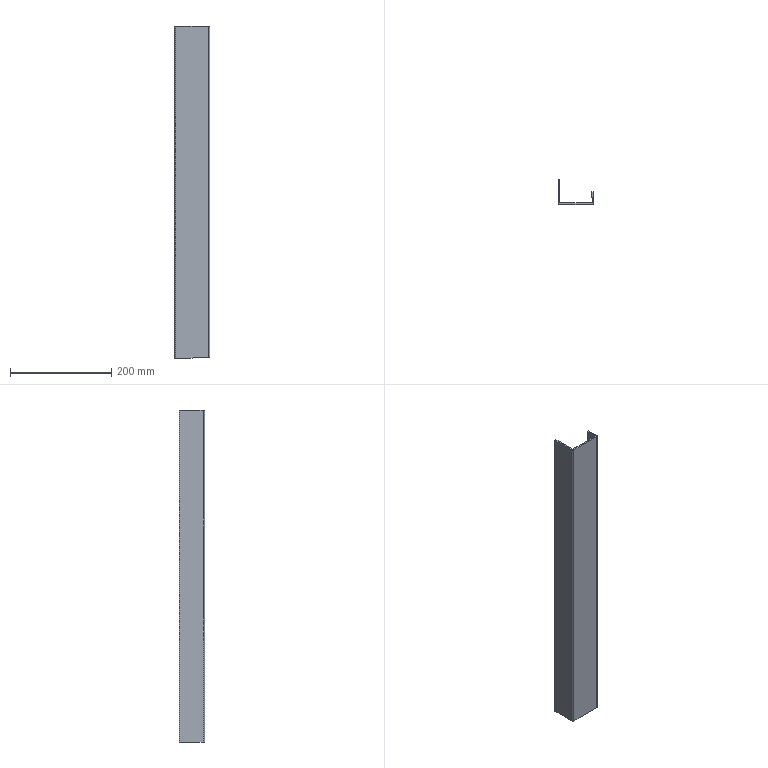Part | SolidWorks | 1 solid | 22 faces | box 69.995 x 50 x 656 mm | volume 270732 mm3 | plane 18 | cylinder 4 | commonest cylinder face diameters 0.2 x2 6.2 x2
STEP:
#1=CARTESIAN_POINT('',(31.895,-3.,-328.));
#2=VERTEX_POINT('',#1);
#3=CARTESIAN_POINT('',(31.895,-3.,328.));
#4=VERTEX_POINT('',#3);
#5=CARTESIAN_POINT('',(31.895,-3.,-328.));
#6=DIRECTION('',(0.,0.,1.));
#7=VECTOR('',#6,1000.);
#8=LINE('',#5,#7);
#9=EDGE_CURVE('',#2,#4,#8,.T.);
#10=ORIENTED_EDGE('',*,*,#9,.T.);
#11=CARTESIAN_POINT('',(-31.9,-3.,328.));
#12=VERTEX_POINT('',#11);
#13=CARTESIAN_POINT('',(35.,-3.,328.));
#14=DIRECTION('',(1.,0.,0.));
#15=VECTOR('',#14,1000.);
#16=LINE('',#13,#15);
#17=EDGE_CURVE('',#12,#4,#16,.T.);
#18=ORIENTED_EDGE('',*,*,#17,.F.);
#19=CARTESIAN_POINT('',(-31.9,-3.,-328.));
#20=VERTEX_POINT('',#19);
#21=CARTESIAN_POINT('',(-31.9,-3.,328.));
#22=DIRECTION('',(0.,0.,-1.));
#23=VECTOR('',#22,1000.);
#24=LINE('',#21,#23);
#25=EDGE_CURVE('',#12,#20,#24,.T.);
#26=ORIENTED_EDGE('',*,*,#25,.T.);
#27=CARTESIAN_POINT('',(35.,-3.,-328.));
#28=DIRECTION('',(-1.,0.,0.));
#29=VECTOR('',#28,1000.);
#30=LINE('',#27,#29);
#31=EDGE_CURVE('',#2,#20,#30,.T.);
#32=ORIENTED_EDGE('',*,*,#31,.F.);
#33=EDGE_LOOP('',(#10,#18,#26,#32));
#34=FACE_OUTER_BOUND('',#33,.T.);
#35=CARTESIAN_POINT('',(0.,-3.,0.));
#36=DIRECTION('',(0.,1.,0.));
#37=DIRECTION('',(0.,0.,1.));
#38=AXIS2_PLACEMENT_3D('',#35,#36,#37);
#39=PLANE('',#38);
#40=ADVANCED_FACE('',(#34),#39,.F.);
#41=CARTESIAN_POINT('',(-31.9,0.,328.));
#42=VERTEX_POINT('',#41);
#43=CARTESIAN_POINT('',(31.895,0.,328.));
#44=VERTEX_POINT('',#43);
#45=CARTESIAN_POINT('',(35.,0.,328.));
#46=DIRECTION('',(1.,0.,0.));
#47=VECTOR('',#46,1000.);
#48=LINE('',#45,#47);
#49=EDGE_CURVE('',#42,#44,#48,.T.);
#50=ORIENTED_EDGE('',*,*,#49,.T.);
#51=CARTESIAN_POINT('',(31.895,0.,-328.));
#52=VERTEX_POINT('',#51);
#53=CARTESIAN_POINT('',(31.895,0.,-328.));
#54=DIRECTION('',(0.,0.,1.));
#55=VECTOR('',#54,1000.);
#56=LINE('',#53,#55);
#57=EDGE_CURVE('',#52,#44,#56,.T.);
#58=ORIENTED_EDGE('',*,*,#57,.F.);
#59=CARTESIAN_POINT('',(-31.9,0.,-328.));
#60=VERTEX_POINT('',#59);
#61=CARTESIAN_POINT('',(35.,0.,-328.));
#62=DIRECTION('',(-1.,0.,0.));
#63=VECTOR('',#62,1000.);
#64=LINE('',#61,#63);
#65=EDGE_CURVE('',#52,#60,#64,.T.);
#66=ORIENTED_EDGE('',*,*,#65,.T.);
#67=CARTESIAN_POINT('',(-31.9,0.,328.));
#68=DIRECTION('',(0.,0.,-1.));
#69=VECTOR('',#68,1000.);
#70=LINE('',#67,#69);
#71=EDGE_CURVE('',#42,#60,#70,.T.);
#72=ORIENTED_EDGE('',*,*,#71,.F.);
#73=EDGE_LOOP('',(#50,#58,#66,#72));
#74=FACE_OUTER_BOUND('',#73,.T.);
#75=CARTESIAN_POINT('',(0.,0.,0.));
#76=DIRECTION('',(0.,1.,0.));
#77=DIRECTION('',(0.,0.,1.));
#78=AXIS2_PLACEMENT_3D('',#75,#76,#77);
#79=PLANE('',#78);
#80=ADVANCED_FACE('',(#74),#79,.T.);
#81=ORIENTED_EDGE('',*,*,#65,.F.);
#82=CARTESIAN_POINT('',(31.895,0.,-328.));
#83=DIRECTION('',(0.,-1.,0.));
#84=VECTOR('',#83,1000.);
#85=LINE('',#82,#84);
#86=EDGE_CURVE('',#52,#2,#85,.T.);
#87=ORIENTED_EDGE('',*,*,#86,.T.);
#88=ORIENTED_EDGE('',*,*,#31,.T.);
#89=CARTESIAN_POINT('',(-31.9,0.,-328.));
#90=DIRECTION('',(0.,-1.,0.));
#91=VECTOR('',#90,1000.);
#92=LINE('',#89,#91);
#93=EDGE_CURVE('',#60,#20,#92,.T.);
#94=ORIENTED_EDGE('',*,*,#93,.F.);
#95=EDGE_LOOP('',(#81,#87,#88,#94));
#96=FACE_OUTER_BOUND('',#95,.T.);
#97=CARTESIAN_POINT('',(35.,-3.,-328.));
#98=DIRECTION('',(0.,0.,-1.));
#99=DIRECTION('',(-1.,0.,0.));
#100=AXIS2_PLACEMENT_3D('',#97,#98,#99);
#101=PLANE('',#100);
#102=ADVANCED_FACE('',(#96),#101,.T.);
#103=CARTESIAN_POINT('',(31.895,0.,328.));
#104=DIRECTION('',(0.,-1.,0.));
#105=VECTOR('',#104,1000.);
#106=LINE('',#103,#105);
#107=EDGE_CURVE('',#44,#4,#106,.T.);
#108=ORIENTED_EDGE('',*,*,#107,.F.);
#109=ORIENTED_EDGE('',*,*,#49,.F.);
#110=CARTESIAN_POINT('',(-31.9,0.,328.));
#111=DIRECTION('',(0.,-1.,0.));
#112=VECTOR('',#111,1000.);
#113=LINE('',#110,#112);
#114=EDGE_CURVE('',#42,#12,#113,.T.);
#115=ORIENTED_EDGE('',*,*,#114,.T.);
#116=ORIENTED_EDGE('',*,*,#17,.T.);
#117=EDGE_LOOP('',(#108,#109,#115,#116));
#118=FACE_OUTER_BOUND('',#117,.T.);
#119=CARTESIAN_POINT('',(35.,-3.,328.));
#120=DIRECTION('',(0.,0.,1.));
#121=DIRECTION('',(1.,0.,0.));
#122=AXIS2_PLACEMENT_3D('',#119,#120,#121);
#123=PLANE('',#122);
#124=ADVANCED_FACE('',(#118),#123,.T.);
#125=CARTESIAN_POINT('',(-32.,0.1,-328.));
#126=VERTEX_POINT('',#125);
#127=CARTESIAN_POINT('',(-35.,0.1,-328.));
#128=VERTEX_POINT('',#127);
#129=CARTESIAN_POINT('',(-35.,0.1,-328.));
#130=DIRECTION('',(-1.,0.,0.));
#131=VECTOR('',#130,1000.);
#132=LINE('',#129,#131);
#133=EDGE_CURVE('',#126,#128,#132,.T.);
#134=ORIENTED_EDGE('',*,*,#133,.F.);
#135=CARTESIAN_POINT('',(-31.9,0.1,-328.));
#136=DIRECTION('',(0.,0.,-1.));
#137=DIRECTION('',(1.,0.,0.));
#138=AXIS2_PLACEMENT_3D('',#135,#136,#137);
#139=CIRCLE('',#138,0.1);
#140=EDGE_CURVE('',#60,#126,#139,.T.);
#141=ORIENTED_EDGE('',*,*,#140,.F.);
#142=ORIENTED_EDGE('',*,*,#93,.T.);
#143=CARTESIAN_POINT('',(-31.9,0.1,-328.));
#144=DIRECTION('',(0.,0.,-1.));
#145=DIRECTION('',(1.,0.,0.));
#146=AXIS2_PLACEMENT_3D('',#143,#144,#145);
#147=CIRCLE('',#146,3.1);
#148=EDGE_CURVE('',#20,#128,#147,.T.);
#149=ORIENTED_EDGE('',*,*,#148,.T.);
#150=EDGE_LOOP('',(#134,#141,#142,#149));
#151=FACE_OUTER_BOUND('',#150,.T.);
#152=CARTESIAN_POINT('',(-31.9,0.1,-328.));
#153=DIRECTION('',(0.,0.,-1.));
#154=DIRECTION('',(-1.,0.,0.));
#155=AXIS2_PLACEMENT_3D('',#152,#153,#154);
#156=PLANE('',#155);
#157=ADVANCED_FACE('',(#151),#156,.T.);
#158=CARTESIAN_POINT('',(-32.,0.1,328.));
#159=VERTEX_POINT('',#158);
#160=CARTESIAN_POINT('',(-31.9,0.1,328.));
#161=DIRECTION('',(0.,0.,1.));
#162=DIRECTION('',(1.,0.,0.));
#163=AXIS2_PLACEMENT_3D('',#160,#161,#162);
#164=CIRCLE('',#163,0.1);
#165=EDGE_CURVE('',#159,#42,#164,.T.);
#166=ORIENTED_EDGE('',*,*,#165,.F.);
#167=CARTESIAN_POINT('',(-35.,0.1,328.));
#168=VERTEX_POINT('',#167);
#169=CARTESIAN_POINT('',(-32.,0.1,328.));
#170=DIRECTION('',(-1.,0.,0.));
#171=VECTOR('',#170,1000.);
#172=LINE('',#169,#171);
#173=EDGE_CURVE('',#159,#168,#172,.T.);
#174=ORIENTED_EDGE('',*,*,#173,.T.);
#175=CARTESIAN_POINT('',(-31.9,0.1,328.));
#176=DIRECTION('',(0.,0.,1.));
#177=DIRECTION('',(1.,0.,0.));
#178=AXIS2_PLACEMENT_3D('',#175,#176,#177);
#179=CIRCLE('',#178,3.1);
#180=EDGE_CURVE('',#168,#12,#179,.T.);
#181=ORIENTED_EDGE('',*,*,#180,.T.);
#182=ORIENTED_EDGE('',*,*,#114,.F.);
#183=EDGE_LOOP('',(#166,#174,#181,#182));
#184=FACE_OUTER_BOUND('',#183,.T.);
#185=CARTESIAN_POINT('',(-31.9,0.1,328.));
#186=DIRECTION('',(0.,0.,-1.));
#187=DIRECTION('',(-1.,0.,0.));
#188=AXIS2_PLACEMENT_3D('',#185,#186,#187);
#189=PLANE('',#188);
#190=ADVANCED_FACE('',(#184),#189,.F.);
#191=ORIENTED_EDGE('',*,*,#25,.F.);
#192=ORIENTED_EDGE('',*,*,#180,.F.);
#193=CARTESIAN_POINT('',(-35.,0.1,-328.));
#194=DIRECTION('',(0.,0.,-1.));
#195=VECTOR('',#194,1000.);
#196=LINE('',#193,#195);
#197=EDGE_CURVE('',#168,#128,#196,.T.);
#198=ORIENTED_EDGE('',*,*,#197,.T.);
#199=ORIENTED_EDGE('',*,*,#148,.F.);
#200=EDGE_LOOP('',(#191,#192,#198,#199));
#201=FACE_OUTER_BOUND('',#200,.T.);
#202=CARTESIAN_POINT('',(-31.9,0.1,328.));
#203=DIRECTION('',(0.,0.,1.));
#204=DIRECTION('',(-1.,0.,0.));
#205=AXIS2_PLACEMENT_3D('',#202,#203,#204);
#206=CYLINDRICAL_SURFACE('',#205,3.1);
#207=ADVANCED_FACE('',(#201),#206,.T.);
#208=ORIENTED_EDGE('',*,*,#71,.T.);
#209=ORIENTED_EDGE('',*,*,#140,.T.);
#210=CARTESIAN_POINT('',(-32.,0.1,-328.));
#211=DIRECTION('',(0.,0.,1.));
#212=VECTOR('',#211,1000.);
#213=LINE('',#210,#212);
#214=EDGE_CURVE('',#126,#159,#213,.T.);
#215=ORIENTED_EDGE('',*,*,#214,.T.);
#216=ORIENTED_EDGE('',*,*,#165,.T.);
#217=EDGE_LOOP('',(#208,#209,#215,#216));
#218=FACE_OUTER_BOUND('',#217,.T.);
#219=CARTESIAN_POINT('',(-31.9,0.1,328.));
#220=DIRECTION('',(0.,0.,1.));
#221=DIRECTION('',(-1.,0.,0.));
#222=AXIS2_PLACEMENT_3D('',#219,#220,#221);
#223=CYLINDRICAL_SURFACE('',#222,0.1);
#224=ADVANCED_FACE('',(#218),#223,.F.);
#225=ORIENTED_EDGE('',*,*,#133,.T.);
#226=CARTESIAN_POINT('',(-35.,47.,-328.));
#227=VERTEX_POINT('',#226);
#228=CARTESIAN_POINT('',(-35.,0.,-328.));
#229=DIRECTION('',(0.,-1.,0.));
#230=VECTOR('',#229,1000.);
#231=LINE('',#228,#230);
#232=EDGE_CURVE('',#227,#128,#231,.T.);
#233=ORIENTED_EDGE('',*,*,#232,.F.);
#234=CARTESIAN_POINT('',(-32.,47.,-328.));
#235=VERTEX_POINT('',#234);
#236=CARTESIAN_POINT('',(-35.,47.,-328.));
#237=DIRECTION('',(1.,0.,0.));
#238=VECTOR('',#237,1000.);
#239=LINE('',#236,#238);
#240=EDGE_CURVE('',#227,#235,#239,.T.);
#241=ORIENTED_EDGE('',*,*,#240,.T.);
#242=CARTESIAN_POINT('',(-32.,0.,-328.));
#243=DIRECTION('',(0.,-1.,0.));
#244=VECTOR('',#243,1000.);
#245=LINE('',#242,#244);
#246=EDGE_CURVE('',#235,#126,#245,.T.);
#247=ORIENTED_EDGE('',*,*,#246,.T.);
#248=EDGE_LOOP('',(#225,#233,#241,#247));
#249=FACE_OUTER_BOUND('',#248,.T.);
#250=CARTESIAN_POINT('',(-35.,0.,-328.));
#251=DIRECTION('',(0.,0.,1.));
#252=DIRECTION('',(1.,0.,0.));
#253=AXIS2_PLACEMENT_3D('',#250,#251,#252);
#254=PLANE('',#253);
#255=ADVANCED_FACE('',(#249),#254,.F.);
#256=ORIENTED_EDGE('',*,*,#173,.F.);
#257=CARTESIAN_POINT('',(-32.,47.,328.));
#258=VERTEX_POINT('',#257);
#259=CARTESIAN_POINT('',(-32.,47.,328.));
#260=DIRECTION('',(0.,1.,0.));
#261=VECTOR('',#260,1000.);
#262=LINE('',#259,#261);
#263=EDGE_CURVE('',#159,#258,#262,.T.);
#264=ORIENTED_EDGE('',*,*,#263,.T.);
#265=CARTESIAN_POINT('',(-35.,47.,328.));
#266=VERTEX_POINT('',#265);
#267=CARTESIAN_POINT('',(-35.,47.,328.));
#268=DIRECTION('',(1.,0.,0.));
#269=VECTOR('',#268,1000.);
#270=LINE('',#267,#269);
#271=EDGE_CURVE('',#266,#258,#270,.T.);
#272=ORIENTED_EDGE('',*,*,#271,.F.);
#273=CARTESIAN_POINT('',(-35.,0.,328.));
#274=DIRECTION('',(0.,1.,0.));
#275=VECTOR('',#274,1000.);
#276=LINE('',#273,#275);
#277=EDGE_CURVE('',#168,#266,#276,.T.);
#278=ORIENTED_EDGE('',*,*,#277,.F.);
#279=EDGE_LOOP('',(#256,#264,#272,#278));
#280=FACE_OUTER_BOUND('',#279,.T.);
#281=CARTESIAN_POINT('',(-35.,47.,328.));
#282=DIRECTION('',(0.,0.,-1.));
#283=DIRECTION('',(0.,1.,0.));
#284=AXIS2_PLACEMENT_3D('',#281,#282,#283);
#285=PLANE('',#284);
#286=ADVANCED_FACE('',(#280),#285,.F.);
#287=ORIENTED_EDGE('',*,*,#197,.F.);
#288=ORIENTED_EDGE('',*,*,#277,.T.);
#289=CARTESIAN_POINT('',(-35.,47.,0.));
#290=DIRECTION('',(0.,0.,-1.));
#291=VECTOR('',#290,1000.);
#292=LINE('',#289,#291);
#293=EDGE_CURVE('',#266,#227,#292,.T.);
#294=ORIENTED_EDGE('',*,*,#293,.T.);
#295=ORIENTED_EDGE('',*,*,#232,.T.);
#296=EDGE_LOOP('',(#287,#288,#294,#295));
#297=FACE_OUTER_BOUND('',#296,.T.);
#298=CARTESIAN_POINT('',(-35.,0.,0.));
#299=DIRECTION('',(1.,0.,0.));
#300=DIRECTION('',(0.,1.,0.));
#301=AXIS2_PLACEMENT_3D('',#298,#299,#300);
#302=PLANE('',#301);
#303=ADVANCED_FACE('',(#297),#302,.F.);
#304=ORIENTED_EDGE('',*,*,#263,.F.);
#305=ORIENTED_EDGE('',*,*,#214,.F.);
#306=ORIENTED_EDGE('',*,*,#246,.F.);
#307=CARTESIAN_POINT('',(-32.,47.,-328.));
#308=DIRECTION('',(0.,0.,-1.));
#309=VECTOR('',#308,1000.);
#310=LINE('',#307,#309);
#311=EDGE_CURVE('',#258,#235,#310,.T.);
#312=ORIENTED_EDGE('',*,*,#311,.F.);
#313=EDGE_LOOP('',(#304,#305,#306,#312));
#314=FACE_OUTER_BOUND('',#313,.T.);
#315=CARTESIAN_POINT('',(-32.,0.,0.));
#316=DIRECTION('',(1.,0.,0.));
#317=DIRECTION('',(0.,1.,0.));
#318=AXIS2_PLACEMENT_3D('',#315,#316,#317);
#319=PLANE('',#318);
#320=ADVANCED_FACE('',(#314),#319,.T.);
#321=ORIENTED_EDGE('',*,*,#311,.T.);
#322=ORIENTED_EDGE('',*,*,#240,.F.);
#323=ORIENTED_EDGE('',*,*,#293,.F.);
#324=ORIENTED_EDGE('',*,*,#271,.T.);
#325=EDGE_LOOP('',(#321,#322,#323,#324));
#326=FACE_OUTER_BOUND('',#325,.T.);
#327=CARTESIAN_POINT('',(-35.,47.,-328.));
#328=DIRECTION('',(0.,-1.,0.));
#329=DIRECTION('',(1.,0.,0.));
#330=AXIS2_PLACEMENT_3D('',#327,#328,#329);
#331=PLANE('',#330);
#332=ADVANCED_FACE('',(#326),#331,.F.);
#333=CARTESIAN_POINT('',(31.995,0.1035,328.));
#334=VERTEX_POINT('',#333);
#335=CARTESIAN_POINT('',(34.993,0.2082,328.));
#336=VERTEX_POINT('',#335);
#337=CARTESIAN_POINT('',(34.993,0.2082,328.));
#338=DIRECTION('',(0.9994,0.0349,0.));
#339=VECTOR('',#338,1000.);
#340=LINE('',#337,#339);
#341=EDGE_CURVE('',#334,#336,#340,.T.);
#342=ORIENTED_EDGE('',*,*,#341,.F.);
#343=CARTESIAN_POINT('',(31.895,0.1,328.));
#344=DIRECTION('',(0.,0.,1.));
#345=DIRECTION('',(-1.,0.,0.));
#346=AXIS2_PLACEMENT_3D('',#343,#344,#345);
#347=CIRCLE('',#346,0.1);
#348=EDGE_CURVE('',#44,#334,#347,.T.);
#349=ORIENTED_EDGE('',*,*,#348,.F.);
#350=ORIENTED_EDGE('',*,*,#107,.T.);
#351=CARTESIAN_POINT('',(31.895,0.1,328.));
#352=DIRECTION('',(0.,0.,1.));
#353=DIRECTION('',(-1.,0.,0.));
#354=AXIS2_PLACEMENT_3D('',#351,#352,#353);
#355=CIRCLE('',#354,3.1);
#356=EDGE_CURVE('',#4,#336,#355,.T.);
#357=ORIENTED_EDGE('',*,*,#356,.T.);
#358=EDGE_LOOP('',(#342,#349,#350,#357));
#359=FACE_OUTER_BOUND('',#358,.T.);
#360=CARTESIAN_POINT('',(31.895,0.1,328.));
#361=DIRECTION('',(0.,0.,1.));
#362=DIRECTION('',(1.,0.,0.));
#363=AXIS2_PLACEMENT_3D('',#360,#361,#362);
#364=PLANE('',#363);
#365=ADVANCED_FACE('',(#359),#364,.T.);
#366=CARTESIAN_POINT('',(31.995,0.1035,-328.));
#367=VERTEX_POINT('',#366);
#368=CARTESIAN_POINT('',(31.895,0.1,-328.));
#369=DIRECTION('',(0.,0.,-1.));
#370=DIRECTION('',(-1.,0.,0.));
#371=AXIS2_PLACEMENT_3D('',#368,#369,#370);
#372=CIRCLE('',#371,0.1);
#373=EDGE_CURVE('',#367,#52,#372,.T.);
#374=ORIENTED_EDGE('',*,*,#373,.F.);
#375=CARTESIAN_POINT('',(34.993,0.2082,-328.));
#376=VERTEX_POINT('',#375);
#377=CARTESIAN_POINT('',(31.995,0.1035,-328.));
#378=DIRECTION('',(0.9994,0.0349,0.));
#379=VECTOR('',#378,1000.);
#380=LINE('',#377,#379);
#381=EDGE_CURVE('',#367,#376,#380,.T.);
#382=ORIENTED_EDGE('',*,*,#381,.T.);
#383=CARTESIAN_POINT('',(31.895,0.1,-328.));
#384=DIRECTION('',(0.,0.,-1.));
#385=DIRECTION('',(-1.,0.,0.));
#386=AXIS2_PLACEMENT_3D('',#383,#384,#385);
#387=CIRCLE('',#386,3.1);
#388=EDGE_CURVE('',#376,#2,#387,.T.);
#389=ORIENTED_EDGE('',*,*,#388,.T.);
#390=ORIENTED_EDGE('',*,*,#86,.F.);
#391=EDGE_LOOP('',(#374,#382,#389,#390));
#392=FACE_OUTER_BOUND('',#391,.T.);
#393=CARTESIAN_POINT('',(31.895,0.1,-328.));
#394=DIRECTION('',(0.,0.,1.));
#395=DIRECTION('',(1.,0.,0.));
#396=AXIS2_PLACEMENT_3D('',#393,#394,#395);
#397=PLANE('',#396);
#398=ADVANCED_FACE('',(#392),#397,.F.);
#399=ORIENTED_EDGE('',*,*,#9,.F.);
#400=ORIENTED_EDGE('',*,*,#388,.F.);
#401=CARTESIAN_POINT('',(34.993,0.2082,328.));
#402=DIRECTION('',(0.,0.,1.));
#403=VECTOR('',#402,1000.);
#404=LINE('',#401,#403);
#405=EDGE_CURVE('',#376,#336,#404,.T.);
#406=ORIENTED_EDGE('',*,*,#405,.T.);
#407=ORIENTED_EDGE('',*,*,#356,.F.);
#408=EDGE_LOOP('',(#399,#400,#406,#407));
#409=FACE_OUTER_BOUND('',#408,.T.);
#410=CARTESIAN_POINT('',(31.895,0.1,-328.));
#411=DIRECTION('',(0.,0.,-1.));
#412=DIRECTION('',(0.9994,0.0349,0.));
#413=AXIS2_PLACEMENT_3D('',#410,#411,#412);
#414=CYLINDRICAL_SURFACE('',#413,3.1);
#415=ADVANCED_FACE('',(#409),#414,.T.);
#416=ORIENTED_EDGE('',*,*,#57,.T.);
#417=ORIENTED_EDGE('',*,*,#348,.T.);
#418=CARTESIAN_POINT('',(31.995,0.1035,328.));
#419=DIRECTION('',(0.,0.,-1.));
#420=VECTOR('',#419,1000.);
#421=LINE('',#418,#420);
#422=EDGE_CURVE('',#334,#367,#421,.T.);
#423=ORIENTED_EDGE('',*,*,#422,.T.);
#424=ORIENTED_EDGE('',*,*,#373,.T.);
#425=EDGE_LOOP('',(#416,#417,#423,#424));
#426=FACE_OUTER_BOUND('',#425,.T.);
#427=CARTESIAN_POINT('',(31.895,0.1,-328.));
#428=DIRECTION('',(0.,0.,-1.));
#429=DIRECTION('',(0.9994,0.0349,0.));
#430=AXIS2_PLACEMENT_3D('',#427,#428,#429);
#431=CYLINDRICAL_SURFACE('',#430,0.1);
#432=ADVANCED_FACE('',(#426),#431,.F.);
#433=ORIENTED_EDGE('',*,*,#381,.F.);
#434=CARTESIAN_POINT('',(31.234,21.88,-328.));
#435=VERTEX_POINT('',#434);
#436=CARTESIAN_POINT('',(31.234,21.88,-328.));
#437=DIRECTION('',(-0.0349,0.9994,0.));
#438=VECTOR('',#437,1000.);
#439=LINE('',#436,#438);
#440=EDGE_CURVE('',#367,#435,#439,.T.);
#441=ORIENTED_EDGE('',*,*,#440,.T.);
#442=CARTESIAN_POINT('',(34.232,21.985,-328.));
#443=VERTEX_POINT('',#442);
#444=CARTESIAN_POINT('',(34.232,21.985,-328.));
#445=DIRECTION('',(-0.9994,-0.0349,0.));
#446=VECTOR('',#445,1000.);
#447=LINE('',#444,#446);
#448=EDGE_CURVE('',#443,#435,#447,.T.);
#449=ORIENTED_EDGE('',*,*,#448,.F.);
#450=CARTESIAN_POINT('',(34.954,1.325,-328.));
#451=DIRECTION('',(-0.0349,0.9994,0.));
#452=VECTOR('',#451,1000.);
#453=LINE('',#450,#452);
#454=EDGE_CURVE('',#376,#443,#453,.T.);
#455=ORIENTED_EDGE('',*,*,#454,.F.);
#456=EDGE_LOOP('',(#433,#441,#449,#455));
#457=FACE_OUTER_BOUND('',#456,.T.);
#458=CARTESIAN_POINT('',(34.232,21.985,-328.));
#459=DIRECTION('',(0.,0.,1.));
#460=DIRECTION('',(0.,-1.,0.));
#461=AXIS2_PLACEMENT_3D('',#458,#459,#460);
#462=PLANE('',#461);
#463=ADVANCED_FACE('',(#457),#462,.F.);
#464=ORIENTED_EDGE('',*,*,#341,.T.);
#465=CARTESIAN_POINT('',(34.232,21.985,328.));
#466=VERTEX_POINT('',#465);
#467=CARTESIAN_POINT('',(34.954,1.325,328.));
#468=DIRECTION('',(0.0349,-0.9994,0.));
#469=VECTOR('',#468,1000.);
#470=LINE('',#467,#469);
#471=EDGE_CURVE('',#466,#336,#470,.T.);
#472=ORIENTED_EDGE('',*,*,#471,.F.);
#473=CARTESIAN_POINT('',(31.234,21.88,328.));
#474=VERTEX_POINT('',#473);
#475=CARTESIAN_POINT('',(34.232,21.985,328.));
#476=DIRECTION('',(-0.9994,-0.0349,0.));
#477=VECTOR('',#476,1000.);
#478=LINE('',#475,#477);
#479=EDGE_CURVE('',#466,#474,#478,.T.);
#480=ORIENTED_EDGE('',*,*,#479,.T.);
#481=CARTESIAN_POINT('',(31.998,0.,328.));
#482=DIRECTION('',(0.0349,-0.9994,0.));
#483=VECTOR('',#482,1000.);
#484=LINE('',#481,#483);
#485=EDGE_CURVE('',#474,#334,#484,.T.);
#486=ORIENTED_EDGE('',*,*,#485,.T.);
#487=EDGE_LOOP('',(#464,#472,#480,#486));
#488=FACE_OUTER_BOUND('',#487,.T.);
#489=CARTESIAN_POINT('',(34.996,0.1047,328.));
#490=DIRECTION('',(0.,0.,-1.));
#491=DIRECTION('',(-1.,0.,0.));
#492=AXIS2_PLACEMENT_3D('',#489,#490,#491);
#493=PLANE('',#492);
#494=ADVANCED_FACE('',(#488),#493,.F.);
#495=ORIENTED_EDGE('',*,*,#405,.F.);
#496=ORIENTED_EDGE('',*,*,#454,.T.);
#497=CARTESIAN_POINT('',(34.232,21.985,0.));
#498=DIRECTION('',(0.,0.,1.));
#499=VECTOR('',#498,1000.);
#500=LINE('',#497,#499);
#501=EDGE_CURVE('',#443,#466,#500,.T.);
#502=ORIENTED_EDGE('',*,*,#501,.T.);
#503=ORIENTED_EDGE('',*,*,#471,.T.);
#504=EDGE_LOOP('',(#495,#496,#502,#503));
#505=FACE_OUTER_BOUND('',#504,.T.);
#506=CARTESIAN_POINT('',(34.954,1.325,0.));
#507=DIRECTION('',(-0.9994,-0.0349,0.));
#508=DIRECTION('',(0.0349,-0.9994,0.));
#509=AXIS2_PLACEMENT_3D('',#506,#507,#508);
#510=PLANE('',#509);
#511=ADVANCED_FACE('',(#505),#510,.F.);
#512=ORIENTED_EDGE('',*,*,#440,.F.);
#513=ORIENTED_EDGE('',*,*,#422,.F.);
#514=ORIENTED_EDGE('',*,*,#485,.F.);
#515=CARTESIAN_POINT('',(31.234,21.88,328.));
#516=DIRECTION('',(0.,0.,1.));
#517=VECTOR('',#516,1000.);
#518=LINE('',#515,#517);
#519=EDGE_CURVE('',#435,#474,#518,.T.);
#520=ORIENTED_EDGE('',*,*,#519,.F.);
#521=EDGE_LOOP('',(#512,#513,#514,#520));
#522=FACE_OUTER_BOUND('',#521,.T.);
#523=CARTESIAN_POINT('',(31.956,1.221,0.));
#524=DIRECTION('',(-0.9994,-0.0349,0.));
#525=DIRECTION('',(0.0349,-0.9994,0.));
#526=AXIS2_PLACEMENT_3D('',#523,#524,#525);
#527=PLANE('',#526);
#528=ADVANCED_FACE('',(#522),#527,.T.);
#529=ORIENTED_EDGE('',*,*,#519,.T.);
#530=ORIENTED_EDGE('',*,*,#479,.F.);
#531=ORIENTED_EDGE('',*,*,#501,.F.);
#532=ORIENTED_EDGE('',*,*,#448,.T.);
#533=EDGE_LOOP('',(#529,#530,#531,#532));
#534=FACE_OUTER_BOUND('',#533,.T.);
#535=CARTESIAN_POINT('',(34.232,21.985,328.));
#536=DIRECTION('',(0.0349,-0.9994,0.));
#537=DIRECTION('',(0.9994,0.0349,0.));
#538=AXIS2_PLACEMENT_3D('',#535,#536,#537);
#539=PLANE('',#538);
#540=ADVANCED_FACE('',(#534),#539,.F.);
#541=CLOSED_SHELL('',(#40,#80,#102,#124,#157,#190,#207,#224,#255,#286,#303,#320,#332,#365,#398,#415,#432,#463,#494,#511,#528,#540));
#542=MANIFOLD_SOLID_BREP('',#541);
#543=CARTESIAN_POINT('',(0.,0.,0.));
#544=DIRECTION('',(0.,0.,1.));
#545=DIRECTION('',(1.,0.,0.));
#546=AXIS2_PLACEMENT_3D('',#543,#544,#545);
#547=(LENGTH_UNIT()NAMED_UNIT(*)SI_UNIT(.MILLI.,.METRE.));
#548=UNCERTAINTY_MEASURE_WITH_UNIT(LENGTH_MEASURE(0.00001),#547,'','');
#549=(NAMED_UNIT(*)PLANE_ANGLE_UNIT()SI_UNIT($,.RADIAN.));
#550=(NAMED_UNIT(*)SI_UNIT($,.STERADIAN.)SOLID_ANGLE_UNIT());
#551=(GEOMETRIC_REPRESENTATION_CONTEXT(3)GLOBAL_UNCERTAINTY_ASSIGNED_CONTEXT((#548))GLOBAL_UNIT_ASSIGNED_CONTEXT((#547,#549,#550))REPRESENTATION_CONTEXT('',''));
#552=ADVANCED_BREP_SHAPE_REPRESENTATION('',(#542,#546),#551);